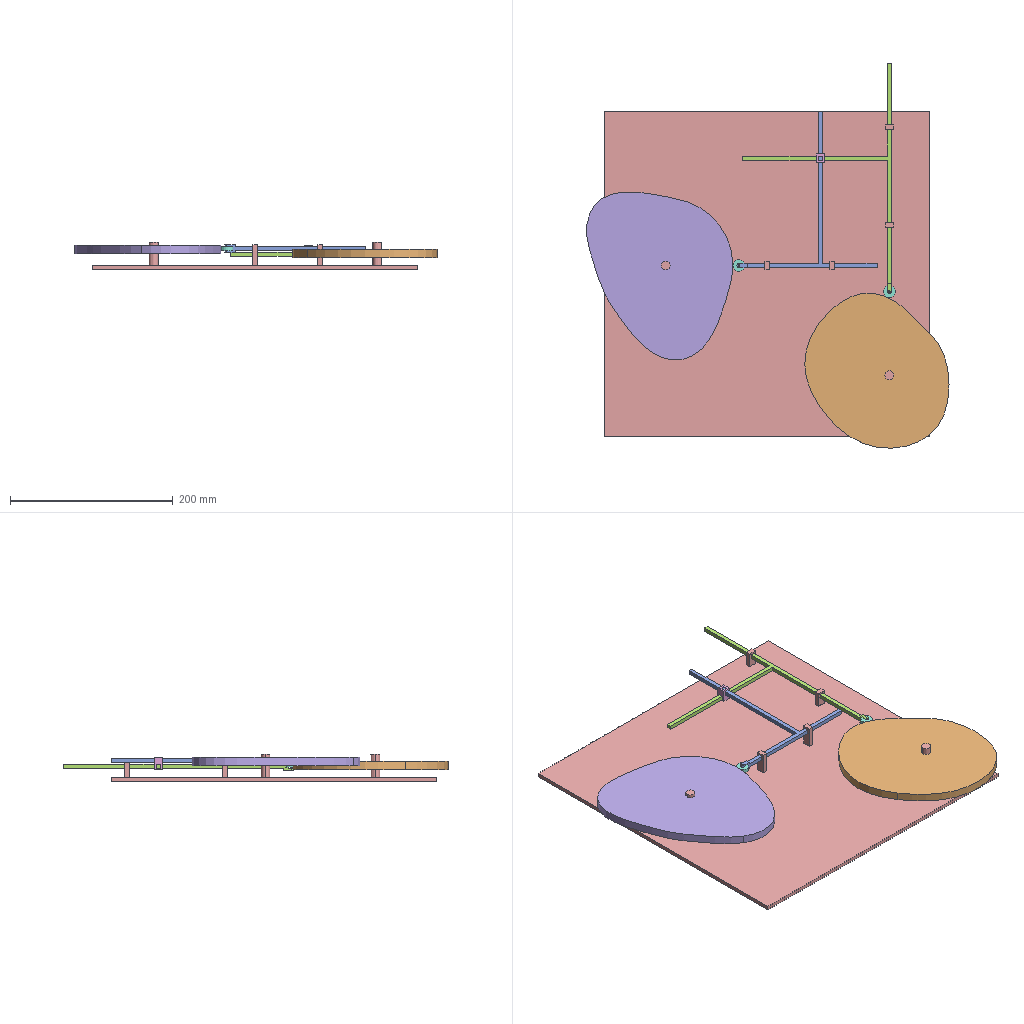Assembly | SolidWorks | 9 different items | 10 placed | box 445 x 473 x 34 mm
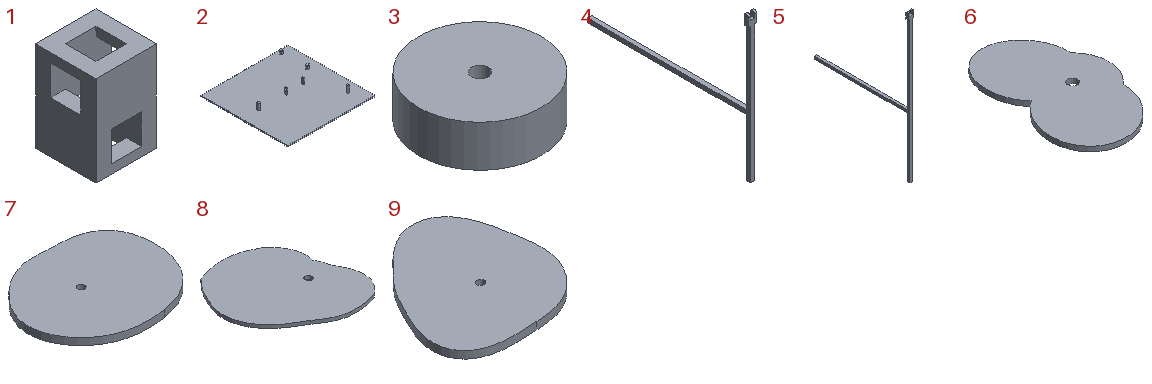Parts list (item | quantity | size | volume | features):
1 | x1 | 10 x 10 x 15 mm | 875 mm3 | features ICE 2, Extrusion 1
2 | x1 | 400 x 400 x 34 mm | 809134 mm3 | features ICE 6, Extrusion 1
3 | x2 | 14.8 x 14.8 x 5 mm | 844.46 mm3 | features Extrusion 1
4 | x1 | 10 x 192.5 x 172.5 mm | 9121 mm3 | features ICE 4, Extrusion 1
5 | x1 | 10 x 182.5 x 282.577 mm | 11623 mm3 | features ICE 4, Extrusion 1
6 | x1 | 95.852 x 152.391 x 5 mm | 53303 mm3 | features CurveInFile 1, Extrusion 1, ICE 1
7 | x1 | 194.935 x 162.289 x 10 mm | 255071 mm3 | features Extrusion 1
8 | x1 | 161.75 x 166.846 x 5 mm | 99438 mm3 | features CurveInFile 1, Extrusion 1, ICE 1
9 | x1 | 185.51 x 198.55 x 10 mm | 275088 mm3 | features Extrusion 1
Mates (type | each side: item.copy, entity, surface, feature):
Coincident | 2.1 face plane Cut-Extrude2 | 4.1 face plane Boss-Extrude1 | 2 times
Coincident | 4.1 edge | 1.1 vertex
Coincident | 2.1 vertex | 5.1 edge
Coincident | 2.1 face plane Cut-Extrude3 | 5.1 face plane Boss-Extrude1
Coincident | 5.1 face plane Boss-Extrude3 | 1.1 face plane Boss-Extrude1
Coincident | 5.1 face plane Boss-Extrude1 | 1.1 face plane Cut-Extrude2
Concentric | 4.1 face cylinder Cut-Extrude2 | 3.1 face cylinder Boss-Extrude1
Coincident | 4.1 face plane Cut-Extrude1 | 3.1 face plane Boss-Extrude1
Concentric | 5.1 face cylinder Cut-Extrude2 | 3.2 face cylinder Boss-Extrude1
Parallel | 5.1 face plane Boss-Extrude1 | 3.2 select_type:24
Parallel | 4.1 face plane Boss-Extrude1 | 3.1 select_type:24
Concentric | 2.1 face cylinder Boss-Extrude7 | 7.1 face cylinder Boss-Extrude1 | 2 times
CamTangent | 7.1 face surface:4009 Boss-Extrude1 | 3.2 face cylinder Boss-Extrude1
DistanceDim | 7.1 face plane Boss-Extrude1 | 2.1 face plane Boss-Extrude1
Concentric | 2.1 edge | 7.1 edge
DistanceDim | 9.1 face plane Boss-Extrude1 | 2.1 face plane Boss-Extrude1
Concentric | 2.1 face cylinder Boss-Extrude7 | 9.1 face cylinder Boss-Extrude1
CamTangent | 9.1 face surface:4009 Boss-Extrude1 | 3.1 face cylinder Boss-Extrude1
GearDim | 9.1 face cylinder Boss-Extrude1 | 7.1 face cylinder Boss-Extrude1